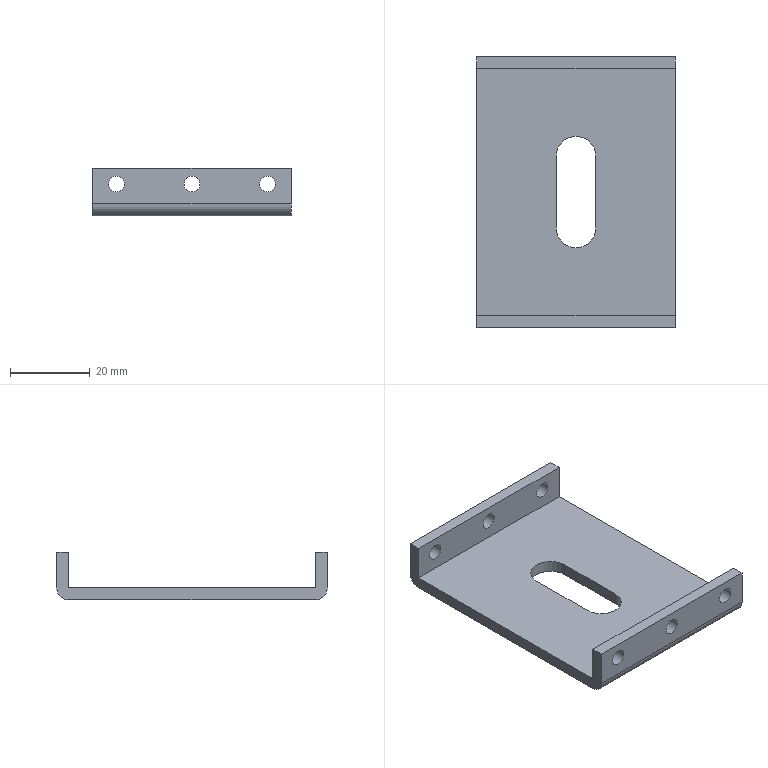Part | STEP file | 1-04.2 | 1 solid | 22 faces | box 50 x 68 x 12 mm | volume 11705 mm3 | plane 12 | cylinder 10 | commonest cylinder face diameters 4 x6 6 x2 10 x2